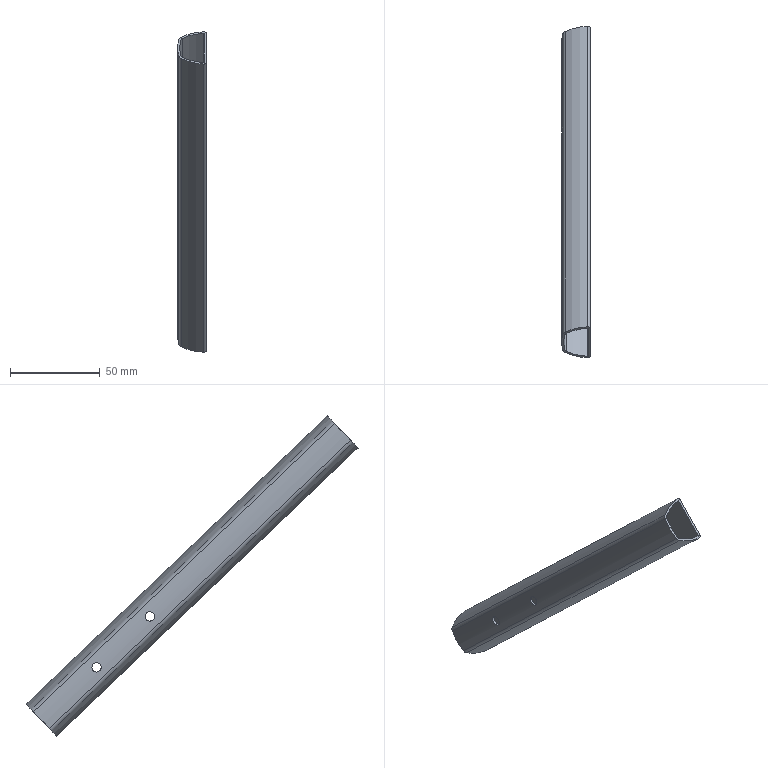Part | SolidWorks | features BaseBody 1 | 1 solid | 34 faces | box 16 x 184.96 x 178.529 mm | volume 18508 mm3 | cylinder 30 | plane 4 | commonest cylinder face diameters 5.2 x8 5.3 x4 0.6 x3 3 x3 3.6 x2 5.5 x2